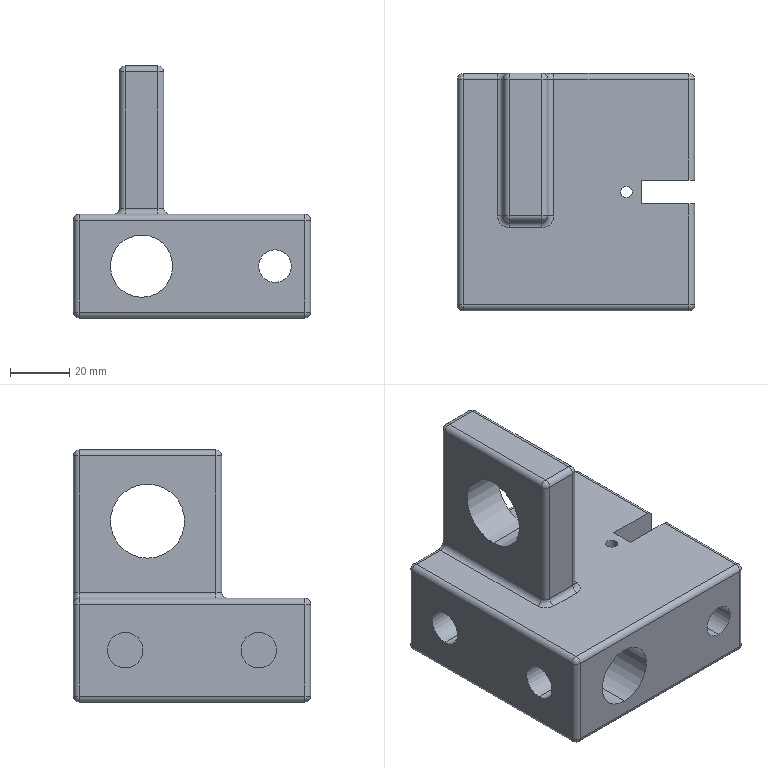Part | SolidWorks | features ICE 5, Extrusion 1, Fillet 1 | 1 solid | 72 faces | box 80 x 80 x 85 mm | volume 211032 mm3 | cylinder 40 | plane 16 | sphere 12 | torus 4 | commonest cylinder face diameters 4 x28 11 x4 12 x4 21 x2 25 x2